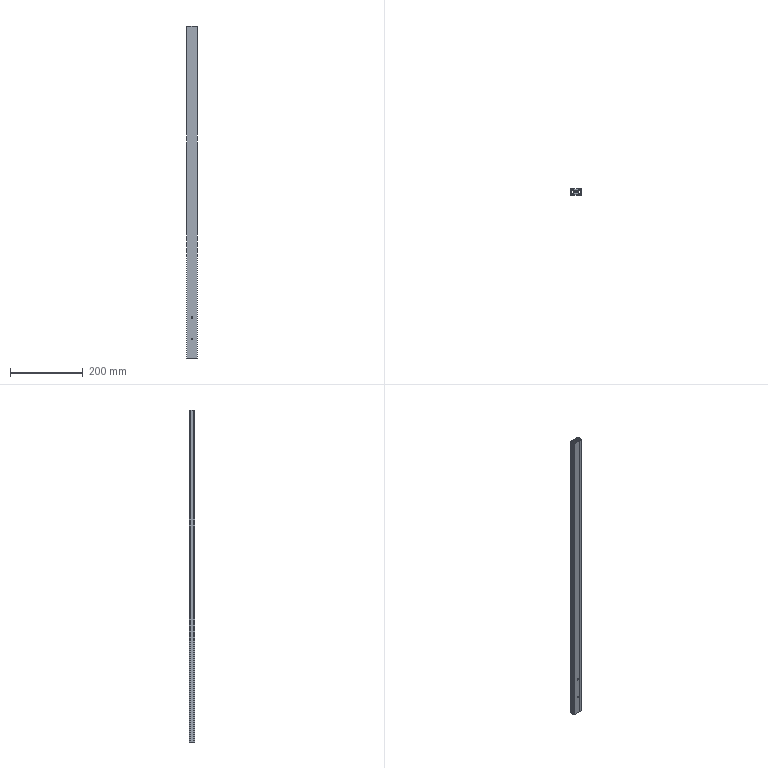Part | SolidWorks | features BaseBody 1, HoleWzd 1, MoveFace 1 | 1 solid | 87 faces | box 30 x 15 x 910 mm | volume 219062 mm3 | plane 46 | cylinder 41 | commonest cylinder face diameters 5 x31 1 x6 2 x4